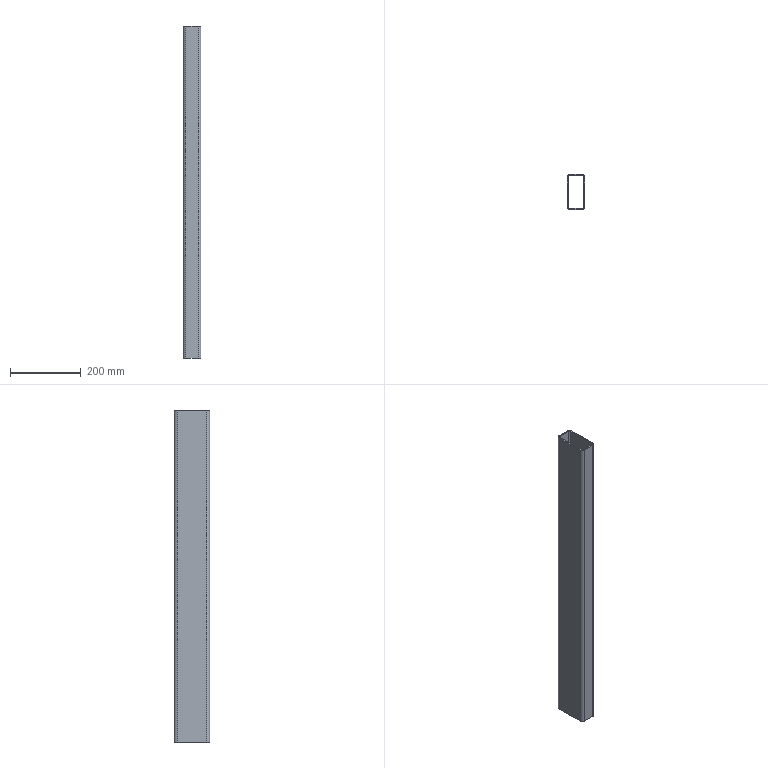Part | STEP file | KS D 3568 - 100 x 50 x 3.2 - 940 | 1 solid | 26 faces | box 50 x 100 x 940 mm | volume 830002 mm3 | cylinder 16 | plane 10 | commonest cylinder face diameters 4.917 x4 9.6 x4 12 x4 16 x4